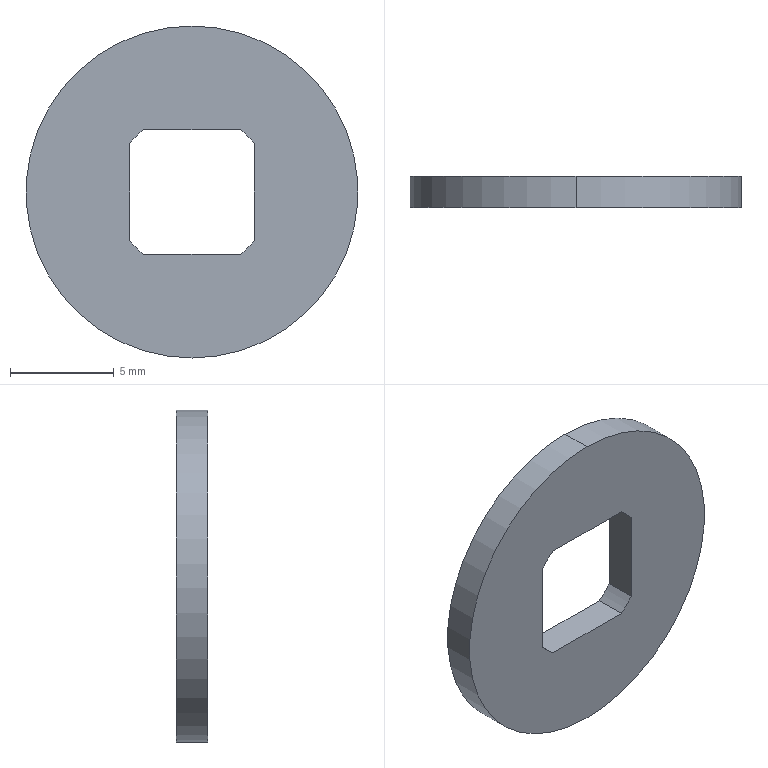Part | SolidWorks | features Extrusion 1 | 1 solid | 12 faces | box 16 x 1.5 x 16 mm | volume 248.819 mm3 | cylinder 6 | plane 6 | commonest cylinder face diameters 7.6 x4 16 x2
STEP:
#1=CARTESIAN_POINT('',(0.,0.,-8.));
#2=VERTEX_POINT('',#1);
#3=CARTESIAN_POINT('',(0.,0.,8.));
#4=VERTEX_POINT('',#3);
#5=CARTESIAN_POINT('',(0.,0.,0.));
#6=DIRECTION('',(0.,-1.,0.));
#7=DIRECTION('',(0.,0.,1.));
#8=AXIS2_PLACEMENT_3D('',#5,#6,#7);
#9=CIRCLE('',#8,8.);
#10=EDGE_CURVE('',#2,#4,#9,.T.);
#11=ORIENTED_EDGE('',*,*,#10,.T.);
#12=CARTESIAN_POINT('',(0.,-1.5,8.));
#13=VERTEX_POINT('',#12);
#14=CARTESIAN_POINT('',(0.,0.,8.));
#15=DIRECTION('',(0.,-1.,0.));
#16=VECTOR('',#15,1000.);
#17=LINE('',#14,#16);
#18=EDGE_CURVE('',#4,#13,#17,.T.);
#19=ORIENTED_EDGE('',*,*,#18,.T.);
#20=CARTESIAN_POINT('',(0.,-1.5,-8.));
#21=VERTEX_POINT('',#20);
#22=CARTESIAN_POINT('',(0.,-1.5,0.));
#23=DIRECTION('',(0.,-1.,0.));
#24=DIRECTION('',(0.,0.,1.));
#25=AXIS2_PLACEMENT_3D('',#22,#23,#24);
#26=CIRCLE('',#25,8.);
#27=EDGE_CURVE('',#21,#13,#26,.T.);
#28=ORIENTED_EDGE('',*,*,#27,.F.);
#29=CARTESIAN_POINT('',(0.,0.,-8.));
#30=DIRECTION('',(0.,-1.,0.));
#31=VECTOR('',#30,1000.);
#32=LINE('',#29,#31);
#33=EDGE_CURVE('',#2,#21,#32,.T.);
#34=ORIENTED_EDGE('',*,*,#33,.F.);
#35=EDGE_LOOP('',(#11,#19,#28,#34));
#36=FACE_OUTER_BOUND('',#35,.T.);
#37=CARTESIAN_POINT('',(0.,0.,0.));
#38=DIRECTION('',(0.,-1.,0.));
#39=DIRECTION('',(0.,0.,-1.));
#40=AXIS2_PLACEMENT_3D('',#37,#38,#39);
#41=CYLINDRICAL_SURFACE('',#40,8.);
#42=ADVANCED_FACE('',(#36),#41,.T.);
#43=ORIENTED_EDGE('',*,*,#18,.F.);
#44=CARTESIAN_POINT('',(0.,0.,0.));
#45=DIRECTION('',(0.,-1.,0.));
#46=DIRECTION('',(0.,0.,1.));
#47=AXIS2_PLACEMENT_3D('',#44,#45,#46);
#48=CIRCLE('',#47,8.);
#49=EDGE_CURVE('',#4,#2,#48,.T.);
#50=ORIENTED_EDGE('',*,*,#49,.T.);
#51=ORIENTED_EDGE('',*,*,#33,.T.);
#52=CARTESIAN_POINT('',(0.,-1.5,0.));
#53=DIRECTION('',(0.,-1.,0.));
#54=DIRECTION('',(0.,0.,1.));
#55=AXIS2_PLACEMENT_3D('',#52,#53,#54);
#56=CIRCLE('',#55,8.);
#57=EDGE_CURVE('',#13,#21,#56,.T.);
#58=ORIENTED_EDGE('',*,*,#57,.F.);
#59=EDGE_LOOP('',(#43,#50,#51,#58));
#60=FACE_OUTER_BOUND('',#59,.T.);
#61=CARTESIAN_POINT('',(0.,0.,0.));
#62=DIRECTION('',(0.,-1.,0.));
#63=DIRECTION('',(0.,0.,-1.));
#64=AXIS2_PLACEMENT_3D('',#61,#62,#63);
#65=CYLINDRICAL_SURFACE('',#64,8.);
#66=ADVANCED_FACE('',(#60),#65,.T.);
#67=CARTESIAN_POINT('',(3.,0.,2.332));
#68=VERTEX_POINT('',#67);
#69=CARTESIAN_POINT('',(2.332,0.,3.));
#70=VERTEX_POINT('',#69);
#71=CARTESIAN_POINT('',(0.,0.,0.));
#72=DIRECTION('',(0.,-1.,0.));
#73=DIRECTION('',(0.,0.,1.));
#74=AXIS2_PLACEMENT_3D('',#71,#72,#73);
#75=CIRCLE('',#74,3.8);
#76=EDGE_CURVE('',#68,#70,#75,.T.);
#77=ORIENTED_EDGE('',*,*,#76,.T.);
#78=CARTESIAN_POINT('',(-2.332,0.,3.));
#79=VERTEX_POINT('',#78);
#80=CARTESIAN_POINT('',(-2.332,0.,3.));
#81=DIRECTION('',(-1.,0.,0.));
#82=VECTOR('',#81,1000.);
#83=LINE('',#80,#82);
#84=EDGE_CURVE('',#70,#79,#83,.T.);
#85=ORIENTED_EDGE('',*,*,#84,.T.);
#86=CARTESIAN_POINT('',(-3.,0.,2.332));
#87=VERTEX_POINT('',#86);
#88=CARTESIAN_POINT('',(0.,0.,0.));
#89=DIRECTION('',(0.,-1.,0.));
#90=DIRECTION('',(0.,0.,1.));
#91=AXIS2_PLACEMENT_3D('',#88,#89,#90);
#92=CIRCLE('',#91,3.8);
#93=EDGE_CURVE('',#79,#87,#92,.T.);
#94=ORIENTED_EDGE('',*,*,#93,.T.);
#95=CARTESIAN_POINT('',(-3.,0.,-2.332));
#96=VERTEX_POINT('',#95);
#97=CARTESIAN_POINT('',(-3.,0.,-2.332));
#98=DIRECTION('',(0.,0.,-1.));
#99=VECTOR('',#98,1000.);
#100=LINE('',#97,#99);
#101=EDGE_CURVE('',#87,#96,#100,.T.);
#102=ORIENTED_EDGE('',*,*,#101,.T.);
#103=CARTESIAN_POINT('',(-2.332,0.,-3.));
#104=VERTEX_POINT('',#103);
#105=CARTESIAN_POINT('',(0.,0.,0.));
#106=DIRECTION('',(0.,-1.,0.));
#107=DIRECTION('',(0.,0.,1.));
#108=AXIS2_PLACEMENT_3D('',#105,#106,#107);
#109=CIRCLE('',#108,3.8);
#110=EDGE_CURVE('',#96,#104,#109,.T.);
#111=ORIENTED_EDGE('',*,*,#110,.T.);
#112=CARTESIAN_POINT('',(2.332,0.,-3.));
#113=VERTEX_POINT('',#112);
#114=CARTESIAN_POINT('',(2.332,0.,-3.));
#115=DIRECTION('',(1.,0.,0.));
#116=VECTOR('',#115,1000.);
#117=LINE('',#114,#116);
#118=EDGE_CURVE('',#104,#113,#117,.T.);
#119=ORIENTED_EDGE('',*,*,#118,.T.);
#120=CARTESIAN_POINT('',(3.,0.,-2.332));
#121=VERTEX_POINT('',#120);
#122=CARTESIAN_POINT('',(0.,0.,0.));
#123=DIRECTION('',(0.,-1.,0.));
#124=DIRECTION('',(0.,0.,1.));
#125=AXIS2_PLACEMENT_3D('',#122,#123,#124);
#126=CIRCLE('',#125,3.8);
#127=EDGE_CURVE('',#113,#121,#126,.T.);
#128=ORIENTED_EDGE('',*,*,#127,.T.);
#129=CARTESIAN_POINT('',(3.,0.,2.332));
#130=DIRECTION('',(0.,0.,1.));
#131=VECTOR('',#130,1000.);
#132=LINE('',#129,#131);
#133=EDGE_CURVE('',#121,#68,#132,.T.);
#134=ORIENTED_EDGE('',*,*,#133,.T.);
#135=EDGE_LOOP('',(#77,#85,#94,#102,#111,#119,#128,#134));
#136=FACE_BOUND('',#135,.T.);
#137=ORIENTED_EDGE('',*,*,#10,.F.);
#138=ORIENTED_EDGE('',*,*,#49,.F.);
#139=EDGE_LOOP('',(#137,#138));
#140=FACE_OUTER_BOUND('',#139,.T.);
#141=CARTESIAN_POINT('',(0.,0.,0.));
#142=DIRECTION('',(0.,1.,0.));
#143=DIRECTION('',(0.,0.,1.));
#144=AXIS2_PLACEMENT_3D('',#141,#142,#143);
#145=PLANE('',#144);
#146=ADVANCED_FACE('',(#136,#140),#145,.T.);
#147=CARTESIAN_POINT('',(2.332,-1.5,3.));
#148=VERTEX_POINT('',#147);
#149=CARTESIAN_POINT('',(-2.332,-1.5,3.));
#150=VERTEX_POINT('',#149);
#151=CARTESIAN_POINT('',(-2.332,-1.5,3.));
#152=DIRECTION('',(-1.,0.,0.));
#153=VECTOR('',#152,1000.);
#154=LINE('',#151,#153);
#155=EDGE_CURVE('',#148,#150,#154,.T.);
#156=ORIENTED_EDGE('',*,*,#155,.F.);
#157=CARTESIAN_POINT('',(3.,-1.5,2.332));
#158=VERTEX_POINT('',#157);
#159=CARTESIAN_POINT('',(0.,-1.5,0.));
#160=DIRECTION('',(0.,-1.,0.));
#161=DIRECTION('',(0.,0.,1.));
#162=AXIS2_PLACEMENT_3D('',#159,#160,#161);
#163=CIRCLE('',#162,3.8);
#164=EDGE_CURVE('',#158,#148,#163,.T.);
#165=ORIENTED_EDGE('',*,*,#164,.F.);
#166=CARTESIAN_POINT('',(3.,-1.5,-2.332));
#167=VERTEX_POINT('',#166);
#168=CARTESIAN_POINT('',(3.,-1.5,2.332));
#169=DIRECTION('',(0.,0.,1.));
#170=VECTOR('',#169,1000.);
#171=LINE('',#168,#170);
#172=EDGE_CURVE('',#167,#158,#171,.T.);
#173=ORIENTED_EDGE('',*,*,#172,.F.);
#174=CARTESIAN_POINT('',(2.332,-1.5,-3.));
#175=VERTEX_POINT('',#174);
#176=CARTESIAN_POINT('',(0.,-1.5,0.));
#177=DIRECTION('',(0.,-1.,0.));
#178=DIRECTION('',(0.,0.,1.));
#179=AXIS2_PLACEMENT_3D('',#176,#177,#178);
#180=CIRCLE('',#179,3.8);
#181=EDGE_CURVE('',#175,#167,#180,.T.);
#182=ORIENTED_EDGE('',*,*,#181,.F.);
#183=CARTESIAN_POINT('',(-2.332,-1.5,-3.));
#184=VERTEX_POINT('',#183);
#185=CARTESIAN_POINT('',(2.332,-1.5,-3.));
#186=DIRECTION('',(1.,0.,0.));
#187=VECTOR('',#186,1000.);
#188=LINE('',#185,#187);
#189=EDGE_CURVE('',#184,#175,#188,.T.);
#190=ORIENTED_EDGE('',*,*,#189,.F.);
#191=CARTESIAN_POINT('',(-3.,-1.5,-2.332));
#192=VERTEX_POINT('',#191);
#193=CARTESIAN_POINT('',(0.,-1.5,0.));
#194=DIRECTION('',(0.,-1.,0.));
#195=DIRECTION('',(0.,0.,1.));
#196=AXIS2_PLACEMENT_3D('',#193,#194,#195);
#197=CIRCLE('',#196,3.8);
#198=EDGE_CURVE('',#192,#184,#197,.T.);
#199=ORIENTED_EDGE('',*,*,#198,.F.);
#200=CARTESIAN_POINT('',(-3.,-1.5,2.332));
#201=VERTEX_POINT('',#200);
#202=CARTESIAN_POINT('',(-3.,-1.5,-2.332));
#203=DIRECTION('',(0.,0.,-1.));
#204=VECTOR('',#203,1000.);
#205=LINE('',#202,#204);
#206=EDGE_CURVE('',#201,#192,#205,.T.);
#207=ORIENTED_EDGE('',*,*,#206,.F.);
#208=CARTESIAN_POINT('',(0.,-1.5,0.));
#209=DIRECTION('',(0.,-1.,0.));
#210=DIRECTION('',(0.,0.,1.));
#211=AXIS2_PLACEMENT_3D('',#208,#209,#210);
#212=CIRCLE('',#211,3.8);
#213=EDGE_CURVE('',#150,#201,#212,.T.);
#214=ORIENTED_EDGE('',*,*,#213,.F.);
#215=EDGE_LOOP('',(#156,#165,#173,#182,#190,#199,#207,#214));
#216=FACE_BOUND('',#215,.T.);
#217=ORIENTED_EDGE('',*,*,#27,.T.);
#218=ORIENTED_EDGE('',*,*,#57,.T.);
#219=EDGE_LOOP('',(#217,#218));
#220=FACE_OUTER_BOUND('',#219,.T.);
#221=CARTESIAN_POINT('',(0.,-1.5,0.));
#222=DIRECTION('',(0.,1.,0.));
#223=DIRECTION('',(0.,0.,1.));
#224=AXIS2_PLACEMENT_3D('',#221,#222,#223);
#225=PLANE('',#224);
#226=ADVANCED_FACE('',(#216,#220),#225,.F.);
#227=ORIENTED_EDGE('',*,*,#164,.T.);
#228=CARTESIAN_POINT('',(2.332,0.,3.));
#229=DIRECTION('',(0.,-1.,0.));
#230=VECTOR('',#229,1000.);
#231=LINE('',#228,#230);
#232=EDGE_CURVE('',#70,#148,#231,.T.);
#233=ORIENTED_EDGE('',*,*,#232,.F.);
#234=ORIENTED_EDGE('',*,*,#76,.F.);
#235=CARTESIAN_POINT('',(3.,0.,2.332));
#236=DIRECTION('',(0.,-1.,0.));
#237=VECTOR('',#236,1000.);
#238=LINE('',#235,#237);
#239=EDGE_CURVE('',#68,#158,#238,.T.);
#240=ORIENTED_EDGE('',*,*,#239,.T.);
#241=EDGE_LOOP('',(#227,#233,#234,#240));
#242=FACE_OUTER_BOUND('',#241,.T.);
#243=CARTESIAN_POINT('',(0.,0.,0.));
#244=DIRECTION('',(0.,-1.,0.));
#245=DIRECTION('',(0.,0.,-1.));
#246=AXIS2_PLACEMENT_3D('',#243,#244,#245);
#247=CYLINDRICAL_SURFACE('',#246,3.8);
#248=ADVANCED_FACE('',(#242),#247,.F.);
#249=ORIENTED_EDGE('',*,*,#172,.T.);
#250=ORIENTED_EDGE('',*,*,#239,.F.);
#251=ORIENTED_EDGE('',*,*,#133,.F.);
#252=CARTESIAN_POINT('',(3.,0.,-2.332));
#253=DIRECTION('',(0.,-1.,0.));
#254=VECTOR('',#253,1000.);
#255=LINE('',#252,#254);
#256=EDGE_CURVE('',#121,#167,#255,.T.);
#257=ORIENTED_EDGE('',*,*,#256,.T.);
#258=EDGE_LOOP('',(#249,#250,#251,#257));
#259=FACE_OUTER_BOUND('',#258,.T.);
#260=CARTESIAN_POINT('',(3.,0.,2.332));
#261=DIRECTION('',(1.,0.,0.));
#262=DIRECTION('',(0.,0.,-1.));
#263=AXIS2_PLACEMENT_3D('',#260,#261,#262);
#264=PLANE('',#263);
#265=ADVANCED_FACE('',(#259),#264,.F.);
#266=ORIENTED_EDGE('',*,*,#181,.T.);
#267=ORIENTED_EDGE('',*,*,#256,.F.);
#268=ORIENTED_EDGE('',*,*,#127,.F.);
#269=CARTESIAN_POINT('',(2.332,0.,-3.));
#270=DIRECTION('',(0.,-1.,0.));
#271=VECTOR('',#270,1000.);
#272=LINE('',#269,#271);
#273=EDGE_CURVE('',#113,#175,#272,.T.);
#274=ORIENTED_EDGE('',*,*,#273,.T.);
#275=EDGE_LOOP('',(#266,#267,#268,#274));
#276=FACE_OUTER_BOUND('',#275,.T.);
#277=CARTESIAN_POINT('',(0.,0.,0.));
#278=DIRECTION('',(0.,-1.,0.));
#279=DIRECTION('',(0.,0.,-1.));
#280=AXIS2_PLACEMENT_3D('',#277,#278,#279);
#281=CYLINDRICAL_SURFACE('',#280,3.8);
#282=ADVANCED_FACE('',(#276),#281,.F.);
#283=ORIENTED_EDGE('',*,*,#189,.T.);
#284=ORIENTED_EDGE('',*,*,#273,.F.);
#285=ORIENTED_EDGE('',*,*,#118,.F.);
#286=CARTESIAN_POINT('',(-2.332,0.,-3.));
#287=DIRECTION('',(0.,-1.,0.));
#288=VECTOR('',#287,1000.);
#289=LINE('',#286,#288);
#290=EDGE_CURVE('',#104,#184,#289,.T.);
#291=ORIENTED_EDGE('',*,*,#290,.T.);
#292=EDGE_LOOP('',(#283,#284,#285,#291));
#293=FACE_OUTER_BOUND('',#292,.T.);
#294=CARTESIAN_POINT('',(2.332,0.,-3.));
#295=DIRECTION('',(0.,0.,-1.));
#296=DIRECTION('',(-1.,0.,0.));
#297=AXIS2_PLACEMENT_3D('',#294,#295,#296);
#298=PLANE('',#297);
#299=ADVANCED_FACE('',(#293),#298,.F.);
#300=ORIENTED_EDGE('',*,*,#198,.T.);
#301=ORIENTED_EDGE('',*,*,#290,.F.);
#302=ORIENTED_EDGE('',*,*,#110,.F.);
#303=CARTESIAN_POINT('',(-3.,0.,-2.332));
#304=DIRECTION('',(0.,-1.,0.));
#305=VECTOR('',#304,1000.);
#306=LINE('',#303,#305);
#307=EDGE_CURVE('',#96,#192,#306,.T.);
#308=ORIENTED_EDGE('',*,*,#307,.T.);
#309=EDGE_LOOP('',(#300,#301,#302,#308));
#310=FACE_OUTER_BOUND('',#309,.T.);
#311=CARTESIAN_POINT('',(0.,0.,0.));
#312=DIRECTION('',(0.,-1.,0.));
#313=DIRECTION('',(0.,0.,-1.));
#314=AXIS2_PLACEMENT_3D('',#311,#312,#313);
#315=CYLINDRICAL_SURFACE('',#314,3.8);
#316=ADVANCED_FACE('',(#310),#315,.F.);
#317=ORIENTED_EDGE('',*,*,#206,.T.);
#318=ORIENTED_EDGE('',*,*,#307,.F.);
#319=ORIENTED_EDGE('',*,*,#101,.F.);
#320=CARTESIAN_POINT('',(-3.,0.,2.332));
#321=DIRECTION('',(0.,-1.,0.));
#322=VECTOR('',#321,1000.);
#323=LINE('',#320,#322);
#324=EDGE_CURVE('',#87,#201,#323,.T.);
#325=ORIENTED_EDGE('',*,*,#324,.T.);
#326=EDGE_LOOP('',(#317,#318,#319,#325));
#327=FACE_OUTER_BOUND('',#326,.T.);
#328=CARTESIAN_POINT('',(-3.,0.,-2.332));
#329=DIRECTION('',(-1.,0.,0.));
#330=DIRECTION('',(0.,0.,1.));
#331=AXIS2_PLACEMENT_3D('',#328,#329,#330);
#332=PLANE('',#331);
#333=ADVANCED_FACE('',(#327),#332,.F.);
#334=ORIENTED_EDGE('',*,*,#213,.T.);
#335=ORIENTED_EDGE('',*,*,#324,.F.);
#336=ORIENTED_EDGE('',*,*,#93,.F.);
#337=CARTESIAN_POINT('',(-2.332,0.,3.));
#338=DIRECTION('',(0.,-1.,0.));
#339=VECTOR('',#338,1000.);
#340=LINE('',#337,#339);
#341=EDGE_CURVE('',#79,#150,#340,.T.);
#342=ORIENTED_EDGE('',*,*,#341,.T.);
#343=EDGE_LOOP('',(#334,#335,#336,#342));
#344=FACE_OUTER_BOUND('',#343,.T.);
#345=CARTESIAN_POINT('',(0.,0.,0.));
#346=DIRECTION('',(0.,-1.,0.));
#347=DIRECTION('',(0.,0.,-1.));
#348=AXIS2_PLACEMENT_3D('',#345,#346,#347);
#349=CYLINDRICAL_SURFACE('',#348,3.8);
#350=ADVANCED_FACE('',(#344),#349,.F.);
#351=ORIENTED_EDGE('',*,*,#155,.T.);
#352=ORIENTED_EDGE('',*,*,#341,.F.);
#353=ORIENTED_EDGE('',*,*,#84,.F.);
#354=ORIENTED_EDGE('',*,*,#232,.T.);
#355=EDGE_LOOP('',(#351,#352,#353,#354));
#356=FACE_OUTER_BOUND('',#355,.T.);
#357=CARTESIAN_POINT('',(-2.332,0.,3.));
#358=DIRECTION('',(0.,0.,1.));
#359=DIRECTION('',(1.,0.,0.));
#360=AXIS2_PLACEMENT_3D('',#357,#358,#359);
#361=PLANE('',#360);
#362=ADVANCED_FACE('',(#356),#361,.F.);
#363=CLOSED_SHELL('',(#42,#66,#146,#226,#248,#265,#282,#299,#316,#333,#350,#362));
#364=MANIFOLD_SOLID_BREP('',#363);
#365=CARTESIAN_POINT('',(0.,0.,0.));
#366=DIRECTION('',(0.,0.,1.));
#367=DIRECTION('',(1.,0.,0.));
#368=AXIS2_PLACEMENT_3D('',#365,#366,#367);
#369=(LENGTH_UNIT()NAMED_UNIT(*)SI_UNIT(.MILLI.,.METRE.));
#370=UNCERTAINTY_MEASURE_WITH_UNIT(LENGTH_MEASURE(0.00001),#369,'','');
#371=(NAMED_UNIT(*)PLANE_ANGLE_UNIT()SI_UNIT($,.RADIAN.));
#372=(NAMED_UNIT(*)SI_UNIT($,.STERADIAN.)SOLID_ANGLE_UNIT());
#373=(GEOMETRIC_REPRESENTATION_CONTEXT(3)GLOBAL_UNCERTAINTY_ASSIGNED_CONTEXT((#370))GLOBAL_UNIT_ASSIGNED_CONTEXT((#369,#371,#372))REPRESENTATION_CONTEXT('',''));
#374=ADVANCED_BREP_SHAPE_REPRESENTATION('',(#364,#368),#373);